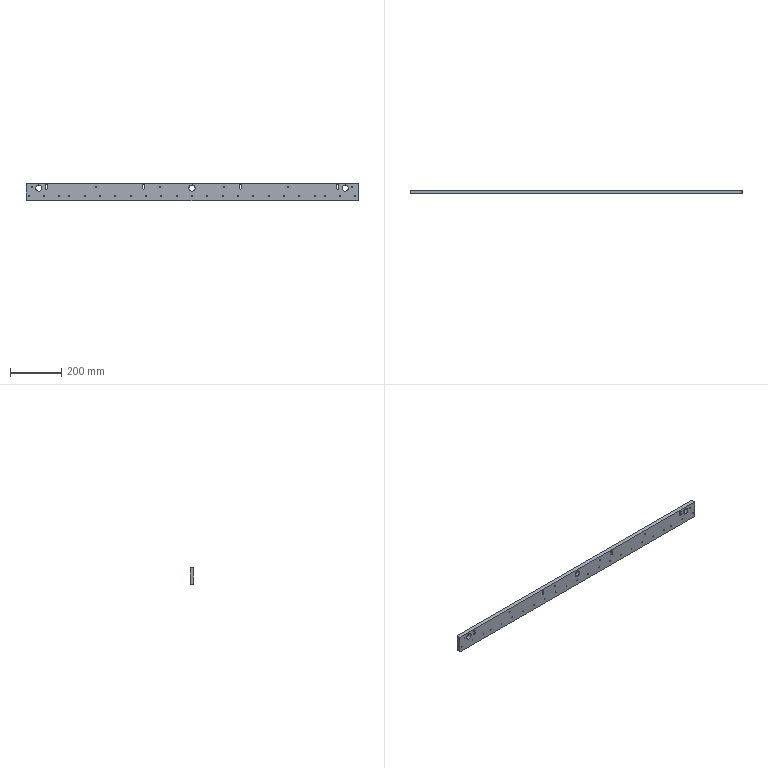Part | NX | features BREP 1 | 1 solid | 122 faces | box 1300 x 15 x 70 mm | volume 1270915 mm3 | cylinder 88 | plane 34 | commonest cylinder face diameters 4.2 x58 10 x12 15 x12 25 x6